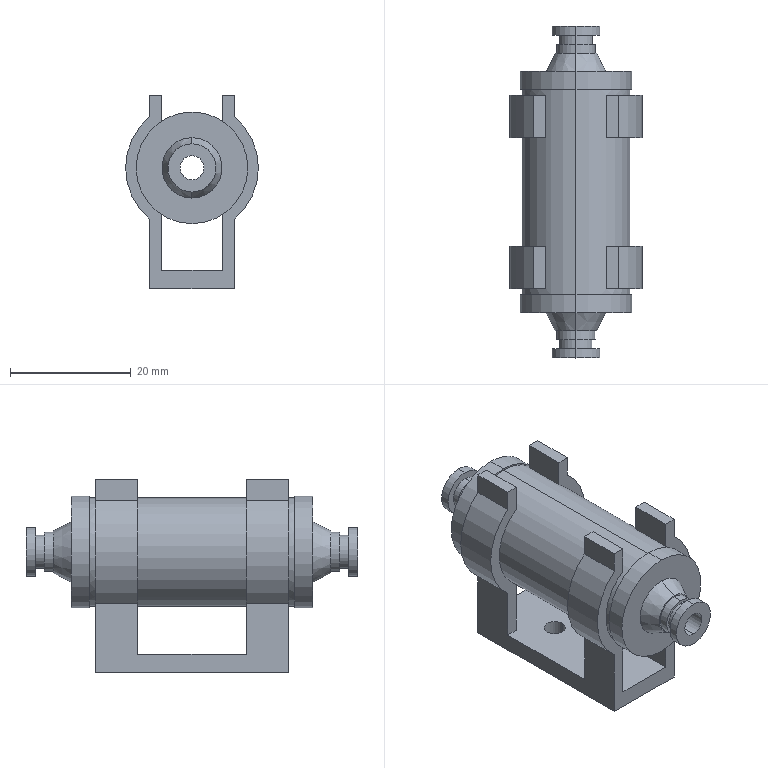Part | SolidWorks | features ICE 3, HoleWzd 2, BaseBody 1 | 1 solid | 70 faces | box 22 x 55 x 32 mm | volume 13292 mm3 | plane 38 | cylinder 28 | cone 4 | commonest cylinder face diameters 3.5 x4 5.5 x4 6.5 x4 8 x4 18.5 x4 22 x4